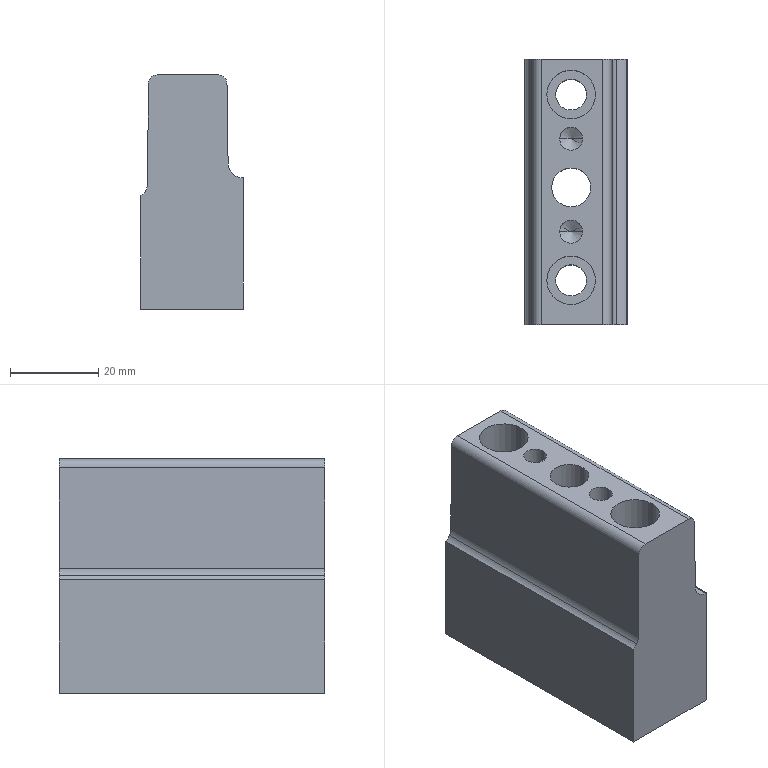Part | 1 solid | 39 faces | box 23.278 x 60 x 52.95 mm | volume 55818 mm3 | cylinder 23 | plane 12 | cone 4 | commonest cylinder face diameters 11 x6 5.2 x4 7 x4 4 x2 6.648 x2 8.8 x2